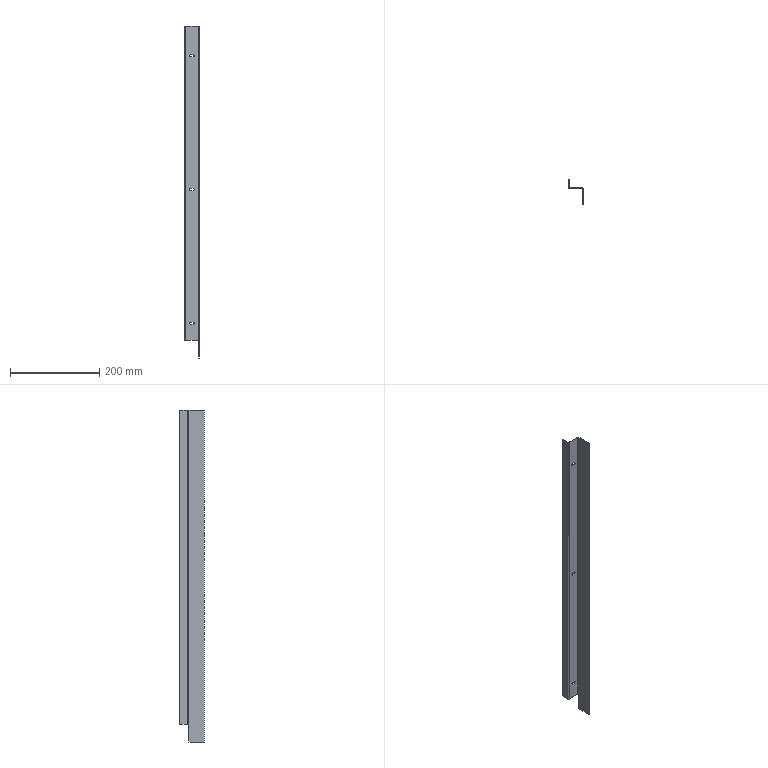Part | NX | features solid 2 | 1 solid | 31 faces | box 32.2 x 56 x 745 mm | volume 73805 mm3 | plane 18 | cylinder 13 | commonest cylinder face diameters 5 x9 2.4 x2 4.8 x2
STEP:
#1=CARTESIAN_POINT('',(1128.5,-1540.,1141.));
#2=VERTEX_POINT('',#1);
#3=CARTESIAN_POINT('',(1128.5,-1538.8,1141.));
#4=VERTEX_POINT('',#3);
#5=CARTESIAN_POINT('',(1128.5,-2286.595,1141.));
#6=DIRECTION('',(0.,1.,0.));
#7=VECTOR('',#6,1000.);
#8=LINE('',#5,#7);
#9=EDGE_CURVE('',#2,#4,#8,.T.);
#10=ORIENTED_EDGE('',*,*,#9,.T.);
#11=CARTESIAN_POINT('',(1123.5,-1538.8,1141.));
#12=VERTEX_POINT('',#11);
#13=CARTESIAN_POINT('',(1128.5,-1538.8,1141.));
#14=DIRECTION('',(-1.,0.,0.));
#15=VECTOR('',#14,1000.);
#16=LINE('',#13,#15);
#17=EDGE_CURVE('',#4,#12,#16,.T.);
#18=ORIENTED_EDGE('',*,*,#17,.T.);
#19=CARTESIAN_POINT('',(1123.5,-1540.,1141.));
#20=VERTEX_POINT('',#19);
#21=CARTESIAN_POINT('',(1123.5,-2286.595,1141.));
#22=DIRECTION('',(0.,1.,0.));
#23=VECTOR('',#22,1000.);
#24=LINE('',#21,#23);
#25=EDGE_CURVE('',#20,#12,#24,.T.);
#26=ORIENTED_EDGE('',*,*,#25,.F.);
#27=CARTESIAN_POINT('',(1141.,-1540.,1141.));
#28=DIRECTION('',(-1.,0.,0.));
#29=VECTOR('',#28,1000.);
#30=LINE('',#27,#29);
#31=EDGE_CURVE('',#2,#20,#30,.T.);
#32=ORIENTED_EDGE('',*,*,#31,.F.);
#33=EDGE_LOOP('',(#10,#18,#26,#32));
#34=FACE_BOUND('',#33,.T.);
#35=CARTESIAN_POINT('',(1128.5,-2286.595,1141.));
#36=DIRECTION('',(0.,0.,-1.));
#37=DIRECTION('',(0.,-1.,0.));
#38=AXIS2_PLACEMENT_3D('',#35,#36,#37);
#39=PLANE('',#38);
#40=ADVANCED_FACE('',(#34),#39,.F.);
#41=CARTESIAN_POINT('',(1128.5,-1540.,1146.));
#42=VERTEX_POINT('',#41);
#43=CARTESIAN_POINT('',(1128.5,-1538.8,1146.));
#44=VERTEX_POINT('',#43);
#45=CARTESIAN_POINT('',(1128.5,-2286.595,1146.));
#46=DIRECTION('',(0.,1.,0.));
#47=VECTOR('',#46,1000.);
#48=LINE('',#45,#47);
#49=EDGE_CURVE('',#42,#44,#48,.T.);
#50=ORIENTED_EDGE('',*,*,#49,.T.);
#51=CARTESIAN_POINT('',(1128.5,-1538.8,1143.5));
#52=DIRECTION('',(0.,1.,0.));
#53=DIRECTION('',(-1.,0.,0.));
#54=AXIS2_PLACEMENT_3D('',#51,#52,#53);
#55=CIRCLE('',#54,2.5);
#56=EDGE_CURVE('',#44,#4,#55,.T.);
#57=ORIENTED_EDGE('',*,*,#56,.T.);
#58=ORIENTED_EDGE('',*,*,#9,.F.);
#59=CARTESIAN_POINT('',(1128.5,-1540.,1143.5));
#60=DIRECTION('',(0.,1.,0.));
#61=DIRECTION('',(-1.,0.,0.));
#62=AXIS2_PLACEMENT_3D('',#59,#60,#61);
#63=CIRCLE('',#62,2.5);
#64=EDGE_CURVE('',#42,#2,#63,.T.);
#65=ORIENTED_EDGE('',*,*,#64,.F.);
#66=EDGE_LOOP('',(#50,#57,#58,#65));
#67=FACE_BOUND('',#66,.T.);
#68=CARTESIAN_POINT('',(1128.5,-2286.595,1143.5));
#69=DIRECTION('',(0.,1.,0.));
#70=DIRECTION('',(-1.,0.,0.));
#71=AXIS2_PLACEMENT_3D('',#68,#69,#70);
#72=CYLINDRICAL_SURFACE('',#71,2.5);
#73=ADVANCED_FACE('',(#67),#72,.F.);
#74=CARTESIAN_POINT('',(1123.5,-1540.,1146.));
#75=VERTEX_POINT('',#74);
#76=CARTESIAN_POINT('',(1123.5,-1538.8,1146.));
#77=VERTEX_POINT('',#76);
#78=CARTESIAN_POINT('',(1123.5,-2286.595,1146.));
#79=DIRECTION('',(0.,1.,0.));
#80=VECTOR('',#79,1000.);
#81=LINE('',#78,#80);
#82=EDGE_CURVE('',#75,#77,#81,.T.);
#83=ORIENTED_EDGE('',*,*,#82,.T.);
#84=CARTESIAN_POINT('',(1128.5,-1538.8,1146.));
#85=DIRECTION('',(1.,0.,0.));
#86=VECTOR('',#85,1000.);
#87=LINE('',#84,#86);
#88=EDGE_CURVE('',#77,#44,#87,.T.);
#89=ORIENTED_EDGE('',*,*,#88,.T.);
#90=ORIENTED_EDGE('',*,*,#49,.F.);
#91=CARTESIAN_POINT('',(1141.,-1540.,1146.));
#92=DIRECTION('',(1.,0.,0.));
#93=VECTOR('',#92,1000.);
#94=LINE('',#91,#93);
#95=EDGE_CURVE('',#75,#42,#94,.T.);
#96=ORIENTED_EDGE('',*,*,#95,.F.);
#97=EDGE_LOOP('',(#83,#89,#90,#96));
#98=FACE_BOUND('',#97,.T.);
#99=CARTESIAN_POINT('',(1128.5,-2286.595,1146.));
#100=DIRECTION('',(0.,0.,1.));
#101=DIRECTION('',(1.,0.,0.));
#102=AXIS2_PLACEMENT_3D('',#99,#100,#101);
#103=PLANE('',#102);
#104=ADVANCED_FACE('',(#98),#103,.F.);
#105=CARTESIAN_POINT('',(1121.,-1540.,1143.5));
#106=VERTEX_POINT('',#105);
#107=CARTESIAN_POINT('',(1121.,-1538.8,1143.5));
#108=VERTEX_POINT('',#107);
#109=CARTESIAN_POINT('',(1121.,-2286.595,1143.5));
#110=DIRECTION('',(0.,1.,0.));
#111=VECTOR('',#110,1000.);
#112=LINE('',#109,#111);
#113=EDGE_CURVE('',#106,#108,#112,.T.);
#114=ORIENTED_EDGE('',*,*,#113,.F.);
#115=CARTESIAN_POINT('',(1123.5,-1540.,1143.5));
#116=DIRECTION('',(0.,1.,0.));
#117=DIRECTION('',(-1.,0.,0.));
#118=AXIS2_PLACEMENT_3D('',#115,#116,#117);
#119=CIRCLE('',#118,2.5);
#120=EDGE_CURVE('',#20,#106,#119,.T.);
#121=ORIENTED_EDGE('',*,*,#120,.F.);
#122=ORIENTED_EDGE('',*,*,#25,.T.);
#123=CARTESIAN_POINT('',(1123.5,-1538.8,1143.5));
#124=DIRECTION('',(0.,1.,0.));
#125=DIRECTION('',(1.,0.,0.));
#126=AXIS2_PLACEMENT_3D('',#123,#124,#125);
#127=CIRCLE('',#126,2.5);
#128=EDGE_CURVE('',#12,#108,#127,.T.);
#129=ORIENTED_EDGE('',*,*,#128,.T.);
#130=EDGE_LOOP('',(#114,#121,#122,#129));
#131=FACE_BOUND('',#130,.T.);
#132=CARTESIAN_POINT('',(1123.5,-2286.595,1143.5));
#133=DIRECTION('',(0.,1.,0.));
#134=DIRECTION('',(-1.,0.,0.));
#135=AXIS2_PLACEMENT_3D('',#132,#133,#134);
#136=CYLINDRICAL_SURFACE('',#135,2.5);
#137=ADVANCED_FACE('',(#131),#136,.F.);
#138=CARTESIAN_POINT('',(1128.5,-1540.,841.));
#139=VERTEX_POINT('',#138);
#140=CARTESIAN_POINT('',(1128.5,-1538.8,841.));
#141=VERTEX_POINT('',#140);
#142=CARTESIAN_POINT('',(1128.5,-2286.595,841.));
#143=DIRECTION('',(0.,1.,0.));
#144=VECTOR('',#143,1000.);
#145=LINE('',#142,#144);
#146=EDGE_CURVE('',#139,#141,#145,.T.);
#147=ORIENTED_EDGE('',*,*,#146,.T.);
#148=CARTESIAN_POINT('',(1123.5,-1538.8,841.));
#149=VERTEX_POINT('',#148);
#150=CARTESIAN_POINT('',(1128.5,-1538.8,841.));
#151=DIRECTION('',(-1.,0.,0.));
#152=VECTOR('',#151,1000.);
#153=LINE('',#150,#152);
#154=EDGE_CURVE('',#141,#149,#153,.T.);
#155=ORIENTED_EDGE('',*,*,#154,.T.);
#156=CARTESIAN_POINT('',(1123.5,-1540.,841.));
#157=VERTEX_POINT('',#156);
#158=CARTESIAN_POINT('',(1123.5,-2286.595,841.));
#159=DIRECTION('',(0.,1.,0.));
#160=VECTOR('',#159,1000.);
#161=LINE('',#158,#160);
#162=EDGE_CURVE('',#157,#149,#161,.T.);
#163=ORIENTED_EDGE('',*,*,#162,.F.);
#164=CARTESIAN_POINT('',(1141.,-1540.,841.));
#165=DIRECTION('',(-1.,0.,0.));
#166=VECTOR('',#165,1000.);
#167=LINE('',#164,#166);
#168=EDGE_CURVE('',#139,#157,#167,.T.);
#169=ORIENTED_EDGE('',*,*,#168,.F.);
#170=EDGE_LOOP('',(#147,#155,#163,#169));
#171=FACE_BOUND('',#170,.T.);
#172=CARTESIAN_POINT('',(1128.5,-2286.595,841.));
#173=DIRECTION('',(0.,0.,-1.));
#174=DIRECTION('',(0.,-1.,0.));
#175=AXIS2_PLACEMENT_3D('',#172,#173,#174);
#176=PLANE('',#175);
#177=ADVANCED_FACE('',(#171),#176,.F.);
#178=CARTESIAN_POINT('',(1128.5,-1540.,846.));
#179=VERTEX_POINT('',#178);
#180=CARTESIAN_POINT('',(1128.5,-1538.8,846.));
#181=VERTEX_POINT('',#180);
#182=CARTESIAN_POINT('',(1128.5,-2286.595,846.));
#183=DIRECTION('',(0.,1.,0.));
#184=VECTOR('',#183,1000.);
#185=LINE('',#182,#184);
#186=EDGE_CURVE('',#179,#181,#185,.T.);
#187=ORIENTED_EDGE('',*,*,#186,.T.);
#188=CARTESIAN_POINT('',(1128.5,-1538.8,843.5));
#189=DIRECTION('',(0.,1.,0.));
#190=DIRECTION('',(0.,0.,1.));
#191=AXIS2_PLACEMENT_3D('',#188,#189,#190);
#192=CIRCLE('',#191,2.5);
#193=EDGE_CURVE('',#181,#141,#192,.T.);
#194=ORIENTED_EDGE('',*,*,#193,.T.);
#195=ORIENTED_EDGE('',*,*,#146,.F.);
#196=CARTESIAN_POINT('',(1128.5,-1540.,843.5));
#197=DIRECTION('',(0.,1.,0.));
#198=DIRECTION('',(-1.,0.,0.));
#199=AXIS2_PLACEMENT_3D('',#196,#197,#198);
#200=CIRCLE('',#199,2.5);
#201=EDGE_CURVE('',#179,#139,#200,.T.);
#202=ORIENTED_EDGE('',*,*,#201,.F.);
#203=EDGE_LOOP('',(#187,#194,#195,#202));
#204=FACE_BOUND('',#203,.T.);
#205=CARTESIAN_POINT('',(1128.5,-2286.595,843.5));
#206=DIRECTION('',(0.,1.,0.));
#207=DIRECTION('',(-1.,0.,0.));
#208=AXIS2_PLACEMENT_3D('',#205,#206,#207);
#209=CYLINDRICAL_SURFACE('',#208,2.5);
#210=ADVANCED_FACE('',(#204),#209,.F.);
#211=CARTESIAN_POINT('',(1123.5,-1540.,846.));
#212=VERTEX_POINT('',#211);
#213=CARTESIAN_POINT('',(1123.5,-1538.8,846.));
#214=VERTEX_POINT('',#213);
#215=CARTESIAN_POINT('',(1123.5,-2286.595,846.));
#216=DIRECTION('',(0.,1.,0.));
#217=VECTOR('',#216,1000.);
#218=LINE('',#215,#217);
#219=EDGE_CURVE('',#212,#214,#218,.T.);
#220=ORIENTED_EDGE('',*,*,#219,.T.);
#221=CARTESIAN_POINT('',(1128.5,-1538.8,846.));
#222=DIRECTION('',(1.,0.,0.));
#223=VECTOR('',#222,1000.);
#224=LINE('',#221,#223);
#225=EDGE_CURVE('',#214,#181,#224,.T.);
#226=ORIENTED_EDGE('',*,*,#225,.T.);
#227=ORIENTED_EDGE('',*,*,#186,.F.);
#228=CARTESIAN_POINT('',(1141.,-1540.,846.));
#229=DIRECTION('',(1.,0.,0.));
#230=VECTOR('',#229,1000.);
#231=LINE('',#228,#230);
#232=EDGE_CURVE('',#212,#179,#231,.T.);
#233=ORIENTED_EDGE('',*,*,#232,.F.);
#234=EDGE_LOOP('',(#220,#226,#227,#233));
#235=FACE_BOUND('',#234,.T.);
#236=CARTESIAN_POINT('',(1128.5,-2286.595,846.));
#237=DIRECTION('',(0.,0.,1.));
#238=DIRECTION('',(1.,0.,0.));
#239=AXIS2_PLACEMENT_3D('',#236,#237,#238);
#240=PLANE('',#239);
#241=ADVANCED_FACE('',(#235),#240,.F.);
#242=CARTESIAN_POINT('',(1121.,-1540.,843.5));
#243=VERTEX_POINT('',#242);
#244=CARTESIAN_POINT('',(1121.,-1538.8,843.5));
#245=VERTEX_POINT('',#244);
#246=CARTESIAN_POINT('',(1121.,-2286.595,843.5));
#247=DIRECTION('',(0.,1.,0.));
#248=VECTOR('',#247,1000.);
#249=LINE('',#246,#248);
#250=EDGE_CURVE('',#243,#245,#249,.T.);
#251=ORIENTED_EDGE('',*,*,#250,.F.);
#252=CARTESIAN_POINT('',(1123.5,-1540.,843.5));
#253=DIRECTION('',(0.,1.,0.));
#254=DIRECTION('',(-1.,0.,0.));
#255=AXIS2_PLACEMENT_3D('',#252,#253,#254);
#256=CIRCLE('',#255,2.5);
#257=EDGE_CURVE('',#157,#243,#256,.T.);
#258=ORIENTED_EDGE('',*,*,#257,.F.);
#259=ORIENTED_EDGE('',*,*,#162,.T.);
#260=CARTESIAN_POINT('',(1123.5,-1538.8,843.5));
#261=DIRECTION('',(0.,1.,0.));
#262=DIRECTION('',(0.,0.,-1.));
#263=AXIS2_PLACEMENT_3D('',#260,#261,#262);
#264=CIRCLE('',#263,2.5);
#265=EDGE_CURVE('',#149,#245,#264,.T.);
#266=ORIENTED_EDGE('',*,*,#265,.T.);
#267=EDGE_LOOP('',(#251,#258,#259,#266));
#268=FACE_BOUND('',#267,.T.);
#269=CARTESIAN_POINT('',(1123.5,-2286.595,843.5));
#270=DIRECTION('',(0.,1.,0.));
#271=DIRECTION('',(-1.,0.,0.));
#272=AXIS2_PLACEMENT_3D('',#269,#270,#271);
#273=CYLINDRICAL_SURFACE('',#272,2.5);
#274=ADVANCED_FACE('',(#268),#273,.F.);
#275=CARTESIAN_POINT('',(1128.5,-1540.,541.));
#276=VERTEX_POINT('',#275);
#277=CARTESIAN_POINT('',(1128.5,-1538.8,541.));
#278=VERTEX_POINT('',#277);
#279=CARTESIAN_POINT('',(1128.5,-2286.595,541.));
#280=DIRECTION('',(0.,1.,0.));
#281=VECTOR('',#280,1000.);
#282=LINE('',#279,#281);
#283=EDGE_CURVE('',#276,#278,#282,.T.);
#284=ORIENTED_EDGE('',*,*,#283,.T.);
#285=CARTESIAN_POINT('',(1123.5,-1538.8,541.));
#286=VERTEX_POINT('',#285);
#287=CARTESIAN_POINT('',(1128.5,-1538.8,541.));
#288=DIRECTION('',(-1.,0.,0.));
#289=VECTOR('',#288,1000.);
#290=LINE('',#287,#289);
#291=EDGE_CURVE('',#278,#286,#290,.T.);
#292=ORIENTED_EDGE('',*,*,#291,.T.);
#293=CARTESIAN_POINT('',(1123.5,-1540.,541.));
#294=VERTEX_POINT('',#293);
#295=CARTESIAN_POINT('',(1123.5,-2286.595,541.));
#296=DIRECTION('',(0.,1.,0.));
#297=VECTOR('',#296,1000.);
#298=LINE('',#295,#297);
#299=EDGE_CURVE('',#294,#286,#298,.T.);
#300=ORIENTED_EDGE('',*,*,#299,.F.);
#301=CARTESIAN_POINT('',(1141.,-1540.,541.));
#302=DIRECTION('',(-1.,0.,0.));
#303=VECTOR('',#302,1000.);
#304=LINE('',#301,#303);
#305=EDGE_CURVE('',#276,#294,#304,.T.);
#306=ORIENTED_EDGE('',*,*,#305,.F.);
#307=EDGE_LOOP('',(#284,#292,#300,#306));
#308=FACE_BOUND('',#307,.T.);
#309=CARTESIAN_POINT('',(1128.5,-2286.595,541.));
#310=DIRECTION('',(0.,0.,-1.));
#311=DIRECTION('',(0.,-1.,0.));
#312=AXIS2_PLACEMENT_3D('',#309,#310,#311);
#313=PLANE('',#312);
#314=ADVANCED_FACE('',(#308),#313,.F.);
#315=CARTESIAN_POINT('',(1128.5,-1540.,546.));
#316=VERTEX_POINT('',#315);
#317=CARTESIAN_POINT('',(1128.5,-1538.8,546.));
#318=VERTEX_POINT('',#317);
#319=CARTESIAN_POINT('',(1128.5,-2286.595,546.));
#320=DIRECTION('',(0.,1.,0.));
#321=VECTOR('',#320,1000.);
#322=LINE('',#319,#321);
#323=EDGE_CURVE('',#316,#318,#322,.T.);
#324=ORIENTED_EDGE('',*,*,#323,.T.);
#325=CARTESIAN_POINT('',(1128.5,-1538.8,543.5));
#326=DIRECTION('',(0.,1.,0.));
#327=DIRECTION('',(-1.,0.,0.));
#328=AXIS2_PLACEMENT_3D('',#325,#326,#327);
#329=CIRCLE('',#328,2.5);
#330=EDGE_CURVE('',#318,#278,#329,.T.);
#331=ORIENTED_EDGE('',*,*,#330,.T.);
#332=ORIENTED_EDGE('',*,*,#283,.F.);
#333=CARTESIAN_POINT('',(1128.5,-1540.,543.5));
#334=DIRECTION('',(0.,1.,0.));
#335=DIRECTION('',(-1.,0.,0.));
#336=AXIS2_PLACEMENT_3D('',#333,#334,#335);
#337=CIRCLE('',#336,2.5);
#338=EDGE_CURVE('',#316,#276,#337,.T.);
#339=ORIENTED_EDGE('',*,*,#338,.F.);
#340=EDGE_LOOP('',(#324,#331,#332,#339));
#341=FACE_BOUND('',#340,.T.);
#342=CARTESIAN_POINT('',(1128.5,-2286.595,543.5));
#343=DIRECTION('',(0.,1.,0.));
#344=DIRECTION('',(-1.,0.,0.));
#345=AXIS2_PLACEMENT_3D('',#342,#343,#344);
#346=CYLINDRICAL_SURFACE('',#345,2.5);
#347=ADVANCED_FACE('',(#341),#346,.F.);
#348=CARTESIAN_POINT('',(1123.5,-1540.,546.));
#349=VERTEX_POINT('',#348);
#350=CARTESIAN_POINT('',(1123.5,-1538.8,546.));
#351=VERTEX_POINT('',#350);
#352=CARTESIAN_POINT('',(1123.5,-2286.595,546.));
#353=DIRECTION('',(0.,1.,0.));
#354=VECTOR('',#353,1000.);
#355=LINE('',#352,#354);
#356=EDGE_CURVE('',#349,#351,#355,.T.);
#357=ORIENTED_EDGE('',*,*,#356,.T.);
#358=CARTESIAN_POINT('',(1128.5,-1538.8,546.));
#359=DIRECTION('',(1.,0.,0.));
#360=VECTOR('',#359,1000.);
#361=LINE('',#358,#360);
#362=EDGE_CURVE('',#351,#318,#361,.T.);
#363=ORIENTED_EDGE('',*,*,#362,.T.);
#364=ORIENTED_EDGE('',*,*,#323,.F.);
#365=CARTESIAN_POINT('',(1141.,-1540.,546.));
#366=DIRECTION('',(1.,0.,0.));
#367=VECTOR('',#366,1000.);
#368=LINE('',#365,#367);
#369=EDGE_CURVE('',#349,#316,#368,.T.);
#370=ORIENTED_EDGE('',*,*,#369,.F.);
#371=EDGE_LOOP('',(#357,#363,#364,#370));
#372=FACE_BOUND('',#371,.T.);
#373=CARTESIAN_POINT('',(1128.5,-2286.595,546.));
#374=DIRECTION('',(0.,0.,1.));
#375=DIRECTION('',(1.,0.,0.));
#376=AXIS2_PLACEMENT_3D('',#373,#374,#375);
#377=PLANE('',#376);
#378=ADVANCED_FACE('',(#372),#377,.F.);
#379=CARTESIAN_POINT('',(1121.,-1540.,543.5));
#380=VERTEX_POINT('',#379);
#381=CARTESIAN_POINT('',(1121.,-1538.8,543.5));
#382=VERTEX_POINT('',#381);
#383=CARTESIAN_POINT('',(1121.,-2286.595,543.5));
#384=DIRECTION('',(0.,1.,0.));
#385=VECTOR('',#384,1000.);
#386=LINE('',#383,#385);
#387=EDGE_CURVE('',#380,#382,#386,.T.);
#388=ORIENTED_EDGE('',*,*,#387,.F.);
#389=CARTESIAN_POINT('',(1123.5,-1540.,543.5));
#390=DIRECTION('',(0.,1.,0.));
#391=DIRECTION('',(-1.,0.,0.));
#392=AXIS2_PLACEMENT_3D('',#389,#390,#391);
#393=CIRCLE('',#392,2.5);
#394=EDGE_CURVE('',#294,#380,#393,.T.);
#395=ORIENTED_EDGE('',*,*,#394,.F.);
#396=ORIENTED_EDGE('',*,*,#299,.T.);
#397=CARTESIAN_POINT('',(1123.5,-1538.8,543.5));
#398=DIRECTION('',(0.,1.,0.));
#399=DIRECTION('',(1.,0.,0.));
#400=AXIS2_PLACEMENT_3D('',#397,#398,#399);
#401=CIRCLE('',#400,2.5);
#402=EDGE_CURVE('',#286,#382,#401,.T.);
#403=ORIENTED_EDGE('',*,*,#402,.T.);
#404=EDGE_LOOP('',(#388,#395,#396,#403));
#405=FACE_BOUND('',#404,.T.);
#406=CARTESIAN_POINT('',(1123.5,-2286.595,543.5));
#407=DIRECTION('',(0.,1.,0.));
#408=DIRECTION('',(-1.,0.,0.));
#409=AXIS2_PLACEMENT_3D('',#406,#407,#408);
#410=CYLINDRICAL_SURFACE('',#409,2.5);
#411=ADVANCED_FACE('',(#405),#410,.F.);
#412=CARTESIAN_POINT('',(1110.,-1537.6,505.5));
#413=VERTEX_POINT('',#412);
#414=CARTESIAN_POINT('',(1110.,-1520.,505.5));
#415=VERTEX_POINT('',#414);
#416=CARTESIAN_POINT('',(1110.,-1540.,505.5));
#417=DIRECTION('',(0.,1.,0.));
#418=VECTOR('',#417,1000.);
#419=LINE('',#416,#418);
#420=EDGE_CURVE('',#413,#415,#419,.T.);
#421=ORIENTED_EDGE('',*,*,#420,.T.);
#422=CARTESIAN_POINT('',(1111.2,-1520.,505.5));
#423=VERTEX_POINT('',#422);
#424=CARTESIAN_POINT('',(1110.,-1520.,505.5));
#425=DIRECTION('',(-1.,0.,0.));
#426=VECTOR('',#425,1000.);
#427=LINE('',#424,#426);
#428=EDGE_CURVE('',#423,#415,#427,.T.);
#429=ORIENTED_EDGE('',*,*,#428,.F.);
#430=CARTESIAN_POINT('',(1111.2,-1537.6,505.5));
#431=VERTEX_POINT('',#430);
#432=CARTESIAN_POINT('',(1111.2,-1540.,505.5));
#433=DIRECTION('',(0.,1.,0.));
#434=VECTOR('',#433,1000.);
#435=LINE('',#432,#434);
#436=EDGE_CURVE('',#431,#423,#435,.T.);
#437=ORIENTED_EDGE('',*,*,#436,.F.);
#438=CARTESIAN_POINT('',(1112.4,-1538.8,505.5));
#439=VERTEX_POINT('',#438);
#440=CARTESIAN_POINT('',(1112.4,-1537.6,505.5));
#441=DIRECTION('',(0.,0.,-1.));
#442=DIRECTION('',(-1.,0.,0.));
#443=AXIS2_PLACEMENT_3D('',#440,#441,#442);
#444=CIRCLE('',#443,1.2);
#445=EDGE_CURVE('',#439,#431,#444,.T.);
#446=ORIENTED_EDGE('',*,*,#445,.F.);
#447=CARTESIAN_POINT('',(1139.8,-1538.8,505.5));
#448=VERTEX_POINT('',#447);
#449=CARTESIAN_POINT('',(1141.,-1538.8,505.5));
#450=DIRECTION('',(-1.,0.,0.));
#451=VECTOR('',#450,1000.);
#452=LINE('',#449,#451);
#453=EDGE_CURVE('',#448,#439,#452,.T.);
#454=ORIENTED_EDGE('',*,*,#453,.F.);
#455=CARTESIAN_POINT('',(1142.2,-1541.2,505.5));
#456=VERTEX_POINT('',#455);
#457=CARTESIAN_POINT('',(1139.8,-1541.2,505.5));
#458=DIRECTION('',(0.,0.,1.));
#459=DIRECTION('',(-1.,0.,0.));
#460=AXIS2_PLACEMENT_3D('',#457,#458,#459);
#461=CIRCLE('',#460,2.4);
#462=EDGE_CURVE('',#456,#448,#461,.T.);
#463=ORIENTED_EDGE('',*,*,#462,.F.);
#464=CARTESIAN_POINT('',(1141.,-1541.2,505.5));
#465=VERTEX_POINT('',#464);
#466=CARTESIAN_POINT('',(1141.,-1541.2,505.5));
#467=DIRECTION('',(-1.,0.,0.));
#468=VECTOR('',#467,1000.);
#469=LINE('',#466,#468);
#470=EDGE_CURVE('',#456,#465,#469,.T.);
#471=ORIENTED_EDGE('',*,*,#470,.T.);
#472=CARTESIAN_POINT('',(1139.8,-1540.,505.5));
#473=VERTEX_POINT('',#472);
#474=CARTESIAN_POINT('',(1139.8,-1541.2,505.5));
#475=DIRECTION('',(0.,0.,1.));
#476=DIRECTION('',(1.,0.,0.));
#477=AXIS2_PLACEMENT_3D('',#474,#475,#476);
#478=CIRCLE('',#477,1.2);
#479=EDGE_CURVE('',#465,#473,#478,.T.);
#480=ORIENTED_EDGE('',*,*,#479,.T.);
#481=CARTESIAN_POINT('',(1112.4,-1540.,505.5));
#482=VERTEX_POINT('',#481);
#483=CARTESIAN_POINT('',(1141.,-1540.,505.5));
#484=DIRECTION('',(-1.,0.,0.));
#485=VECTOR('',#484,1000.);
#486=LINE('',#483,#485);
#487=EDGE_CURVE('',#473,#482,#486,.T.);
#488=ORIENTED_EDGE('',*,*,#487,.T.);
#489=CARTESIAN_POINT('',(1112.4,-1537.6,505.5));
#490=DIRECTION('',(0.,0.,-1.));
#491=DIRECTION('',(1.,0.,0.));
#492=AXIS2_PLACEMENT_3D('',#489,#490,#491);
#493=CIRCLE('',#492,2.4);
#494=EDGE_CURVE('',#482,#413,#493,.T.);
#495=ORIENTED_EDGE('',*,*,#494,.T.);
#496=EDGE_LOOP('',(#421,#429,#437,#446,#454,#463,#471,#480,#488,#495));
#497=FACE_BOUND('',#496,.T.);
#498=CARTESIAN_POINT('',(1110.,-1540.,505.5));
#499=DIRECTION('',(0.,0.,-1.));
#500=DIRECTION('',(0.,-1.,0.));
#501=AXIS2_PLACEMENT_3D('',#498,#499,#500);
#502=PLANE('',#501);
#503=ADVANCED_FACE('',(#497),#502,.T.);
#504=CARTESIAN_POINT('',(1142.2,-1541.2,465.5));
#505=VERTEX_POINT('',#504);
#506=CARTESIAN_POINT('',(1141.,-1541.2,465.5));
#507=VERTEX_POINT('',#506);
#508=CARTESIAN_POINT('',(1141.,-1541.2,465.5));
#509=DIRECTION('',(-1.,0.,0.));
#510=VECTOR('',#509,1000.);
#511=LINE('',#508,#510);
#512=EDGE_CURVE('',#505,#507,#511,.T.);
#513=ORIENTED_EDGE('',*,*,#512,.T.);
#514=CARTESIAN_POINT('',(1141.,-1541.2,465.5));
#515=DIRECTION('',(0.,0.,1.));
#516=VECTOR('',#515,1000.);
#517=LINE('',#514,#516);
#518=EDGE_CURVE('',#507,#465,#517,.T.);
#519=ORIENTED_EDGE('',*,*,#518,.T.);
#520=ORIENTED_EDGE('',*,*,#470,.F.);
#521=CARTESIAN_POINT('',(1142.2,-1541.2,465.5));
#522=DIRECTION('',(0.,0.,1.));
#523=VECTOR('',#522,1000.);
#524=LINE('',#521,#523);
#525=EDGE_CURVE('',#505,#456,#524,.T.);
#526=ORIENTED_EDGE('',*,*,#525,.F.);
#527=EDGE_LOOP('',(#513,#519,#520,#526));
#528=FACE_BOUND('',#527,.T.);
#529=CARTESIAN_POINT('',(1141.,-1541.2,485.5));
#530=DIRECTION('',(0.,1.,0.));
#531=DIRECTION('',(1.,0.,0.));
#532=AXIS2_PLACEMENT_3D('',#529,#530,#531);
#533=PLANE('',#532);
#534=ADVANCED_FACE('',(#528),#533,.T.);
#535=CARTESIAN_POINT('',(1110.,-1520.,1210.5));
#536=VERTEX_POINT('',#535);
#537=CARTESIAN_POINT('',(1110.,-1520.,465.5));
#538=DIRECTION('',(0.,0.,1.));
#539=VECTOR('',#538,1000.);
#540=LINE('',#537,#539);
#541=EDGE_CURVE('',#415,#536,#540,.T.);
#542=ORIENTED_EDGE('',*,*,#541,.F.);
#543=ORIENTED_EDGE('',*,*,#420,.F.);
#544=CARTESIAN_POINT('',(1110.,-1537.6,1210.5));
#545=VERTEX_POINT('',#544);
#546=CARTESIAN_POINT('',(1110.,-1537.6,465.5));
#547=DIRECTION('',(0.,0.,1.));
#548=VECTOR('',#547,1000.);
#549=LINE('',#546,#548);
#550=EDGE_CURVE('',#413,#545,#549,.T.);
#551=ORIENTED_EDGE('',*,*,#550,.T.);
#552=CARTESIAN_POINT('',(1110.,-1540.,1210.5));
#553=DIRECTION('',(0.,1.,0.));
#554=VECTOR('',#553,1000.);
#555=LINE('',#552,#554);
#556=EDGE_CURVE('',#545,#536,#555,.T.);
#557=ORIENTED_EDGE('',*,*,#556,.T.);
#558=EDGE_LOOP('',(#542,#543,#551,#557));
#559=FACE_BOUND('',#558,.T.);
#560=CARTESIAN_POINT('',(1110.,-1540.,465.5));
#561=DIRECTION('',(1.,0.,0.));
#562=DIRECTION('',(0.,0.,1.));
#563=AXIS2_PLACEMENT_3D('',#560,#561,#562);
#564=PLANE('',#563);
#565=ADVANCED_FACE('',(#559),#564,.F.);
#566=ORIENTED_EDGE('',*,*,#550,.F.);
#567=ORIENTED_EDGE('',*,*,#494,.F.);
#568=CARTESIAN_POINT('',(1112.4,-1540.,1210.5));
#569=VERTEX_POINT('',#568);
#570=CARTESIAN_POINT('',(1112.4,-1540.,465.5));
#571=DIRECTION('',(0.,0.,1.));
#572=VECTOR('',#571,1000.);
#573=LINE('',#570,#572);
#574=EDGE_CURVE('',#482,#569,#573,.T.);
#575=ORIENTED_EDGE('',*,*,#574,.T.);
#576=CARTESIAN_POINT('',(1112.4,-1537.6,1210.5));
#577=DIRECTION('',(0.,0.,-1.));
#578=DIRECTION('',(-1.,0.,0.));
#579=AXIS2_PLACEMENT_3D('',#576,#577,#578);
#580=CIRCLE('',#579,2.4);
#581=EDGE_CURVE('',#569,#545,#580,.T.);
#582=ORIENTED_EDGE('',*,*,#581,.T.);
#583=EDGE_LOOP('',(#566,#567,#575,#582));
#584=FACE_BOUND('',#583,.T.);
#585=CARTESIAN_POINT('',(1112.4,-1537.6,465.5));
#586=DIRECTION('',(0.,0.,1.));
#587=DIRECTION('',(-1.,0.,0.));
#588=AXIS2_PLACEMENT_3D('',#585,#586,#587);
#589=CYLINDRICAL_SURFACE('',#588,2.4);
#590=ADVANCED_FACE('',(#584),#589,.T.);
#591=ORIENTED_EDGE('',*,*,#305,.T.);
#592=ORIENTED_EDGE('',*,*,#394,.T.);
#593=CARTESIAN_POINT('',(1123.5,-1540.,543.5));
#594=DIRECTION('',(0.,1.,0.));
#595=DIRECTION('',(-1.,0.,0.));
#596=AXIS2_PLACEMENT_3D('',#593,#594,#595);
#597=CIRCLE('',#596,2.5);
#598=EDGE_CURVE('',#380,#349,#597,.T.);
#599=ORIENTED_EDGE('',*,*,#598,.T.);
#600=ORIENTED_EDGE('',*,*,#369,.T.);
#601=ORIENTED_EDGE('',*,*,#338,.T.);
#602=EDGE_LOOP('',(#591,#592,#599,#600,#601));
#603=FACE_BOUND('',#602,.T.);
#604=ORIENTED_EDGE('',*,*,#168,.T.);
#605=ORIENTED_EDGE('',*,*,#257,.T.);
#606=CARTESIAN_POINT('',(1123.5,-1540.,843.5));
#607=DIRECTION('',(0.,1.,0.));
#608=DIRECTION('',(-1.,0.,0.));
#609=AXIS2_PLACEMENT_3D('',#606,#607,#608);
#610=CIRCLE('',#609,2.5);
#611=EDGE_CURVE('',#243,#212,#610,.T.);
#612=ORIENTED_EDGE('',*,*,#611,.T.);
#613=ORIENTED_EDGE('',*,*,#232,.T.);
#614=ORIENTED_EDGE('',*,*,#201,.T.);
#615=EDGE_LOOP('',(#604,#605,#612,#613,#614));
#616=FACE_BOUND('',#615,.T.);
#617=ORIENTED_EDGE('',*,*,#31,.T.);
#618=ORIENTED_EDGE('',*,*,#120,.T.);
#619=CARTESIAN_POINT('',(1123.5,-1540.,1143.5));
#620=DIRECTION('',(0.,1.,0.));
#621=DIRECTION('',(-1.,0.,0.));
#622=AXIS2_PLACEMENT_3D('',#619,#620,#621);
#623=CIRCLE('',#622,2.5);
#624=EDGE_CURVE('',#106,#75,#623,.T.);
#625=ORIENTED_EDGE('',*,*,#624,.T.);
#626=ORIENTED_EDGE('',*,*,#95,.T.);
#627=ORIENTED_EDGE('',*,*,#64,.T.);
#628=EDGE_LOOP('',(#617,#618,#625,#626,#627));
#629=FACE_BOUND('',#628,.T.);
#630=ORIENTED_EDGE('',*,*,#574,.F.);
#631=ORIENTED_EDGE('',*,*,#487,.F.);
#632=CARTESIAN_POINT('',(1139.8,-1540.,1210.5));
#633=VERTEX_POINT('',#632);
#634=CARTESIAN_POINT('',(1139.8,-1540.,465.5));
#635=DIRECTION('',(0.,0.,1.));
#636=VECTOR('',#635,1000.);
#637=LINE('',#634,#636);
#638=EDGE_CURVE('',#473,#633,#637,.T.);
#639=ORIENTED_EDGE('',*,*,#638,.T.);
#640=CARTESIAN_POINT('',(1141.,-1540.,1210.5));
#641=DIRECTION('',(-1.,0.,0.));
#642=VECTOR('',#641,1000.);
#643=LINE('',#640,#642);
#644=EDGE_CURVE('',#633,#569,#643,.T.);
#645=ORIENTED_EDGE('',*,*,#644,.T.);
#646=EDGE_LOOP('',(#630,#631,#639,#645));
#647=FACE_BOUND('',#646,.T.);
#648=CARTESIAN_POINT('',(1141.,-1540.,465.5));
#649=DIRECTION('',(0.,1.,0.));
#650=DIRECTION('',(1.,0.,0.));
#651=AXIS2_PLACEMENT_3D('',#648,#649,#650);
#652=PLANE('',#651);
#653=ADVANCED_FACE('',(#603,#616,#629,#647),#652,.F.);
#654=ORIENTED_EDGE('',*,*,#638,.F.);
#655=ORIENTED_EDGE('',*,*,#479,.F.);
#656=CARTESIAN_POINT('',(1141.,-1541.2,1210.5));
#657=VERTEX_POINT('',#656);
#658=CARTESIAN_POINT('',(1141.,-1541.2,465.5));
#659=DIRECTION('',(0.,0.,1.));
#660=VECTOR('',#659,1000.);
#661=LINE('',#658,#660);
#662=EDGE_CURVE('',#465,#657,#661,.T.);
#663=ORIENTED_EDGE('',*,*,#662,.T.);
#664=CARTESIAN_POINT('',(1139.8,-1541.2,1210.5));
#665=DIRECTION('',(0.,0.,1.));
#666=DIRECTION('',(1.,0.,0.));
#667=AXIS2_PLACEMENT_3D('',#664,#665,#666);
#668=CIRCLE('',#667,1.2);
#669=EDGE_CURVE('',#657,#633,#668,.T.);
#670=ORIENTED_EDGE('',*,*,#669,.T.);
#671=EDGE_LOOP('',(#654,#655,#663,#670));
#672=FACE_BOUND('',#671,.T.);
#673=CARTESIAN_POINT('',(1139.8,-1541.2,465.5));
#674=DIRECTION('',(0.,0.,1.));
#675=DIRECTION('',(-1.,0.,0.));
#676=AXIS2_PLACEMENT_3D('',#673,#674,#675);
#677=CYLINDRICAL_SURFACE('',#676,1.2);
#678=ADVANCED_FACE('',(#672),#677,.F.);
#679=CARTESIAN_POINT('',(1141.,-1576.,1210.5));
#680=VERTEX_POINT('',#679);
#681=CARTESIAN_POINT('',(1141.,-1576.,1210.5));
#682=DIRECTION('',(0.,1.,0.));
#683=VECTOR('',#682,1000.);
#684=LINE('',#681,#683);
#685=EDGE_CURVE('',#680,#657,#684,.T.);
#686=ORIENTED_EDGE('',*,*,#685,.T.);
#687=ORIENTED_EDGE('',*,*,#662,.F.);
#688=ORIENTED_EDGE('',*,*,#518,.F.);
#689=CARTESIAN_POINT('',(1141.,-1576.,465.5));
#690=VERTEX_POINT('',#689);
#691=CARTESIAN_POINT('',(1141.,-1576.,465.5));
#692=DIRECTION('',(0.,1.,0.));
#693=VECTOR('',#692,1000.);
#694=LINE('',#691,#693);
#695=EDGE_CURVE('',#690,#507,#694,.T.);
#696=ORIENTED_EDGE('',*,*,#695,.F.);
#697=CARTESIAN_POINT('',(1141.,-1576.,465.5));
#698=DIRECTION('',(0.,0.,1.));
#699=VECTOR('',#698,1000.);
#700=LINE('',#697,#699);
#701=EDGE_CURVE('',#690,#680,#700,.T.);
#702=ORIENTED_EDGE('',*,*,#701,.T.);
#703=EDGE_LOOP('',(#686,#687,#688,#696,#702));
#704=FACE_BOUND('',#703,.T.);
#705=CARTESIAN_POINT('',(1141.,-1576.,465.5));
#706=DIRECTION('',(1.,0.,0.));
#707=DIRECTION('',(0.,0.,1.));
#708=AXIS2_PLACEMENT_3D('',#705,#706,#707);
#709=PLANE('',#708);
#710=ADVANCED_FACE('',(#704),#709,.F.);
#711=ORIENTED_EDGE('',*,*,#436,.T.);
#712=CARTESIAN_POINT('',(1111.2,-1520.,1210.5));
#713=VERTEX_POINT('',#712);
#714=CARTESIAN_POINT('',(1111.2,-1520.,465.5));
#715=DIRECTION('',(0.,0.,1.));
#716=VECTOR('',#715,1000.);
#717=LINE('',#714,#716);
#718=EDGE_CURVE('',#423,#713,#717,.T.);
#719=ORIENTED_EDGE('',*,*,#718,.T.);
#720=CARTESIAN_POINT('',(1111.2,-1537.6,1210.5));
#721=VERTEX_POINT('',#720);
#722=CARTESIAN_POINT('',(1111.2,-1540.,1210.5));
#723=DIRECTION('',(0.,1.,0.));
#724=VECTOR('',#723,1000.);
#725=LINE('',#722,#724);
#726=EDGE_CURVE('',#721,#713,#725,.T.);
#727=ORIENTED_EDGE('',*,*,#726,.F.);
#728=CARTESIAN_POINT('',(1111.2,-1537.6,465.5));
#729=DIRECTION('',(0.,0.,1.));
#730=VECTOR('',#729,1000.);
#731=LINE('',#728,#730);
#732=EDGE_CURVE('',#431,#721,#731,.T.);
#733=ORIENTED_EDGE('',*,*,#732,.F.);
#734=EDGE_LOOP('',(#711,#719,#727,#733));
#735=FACE_BOUND('',#734,.T.);
#736=CARTESIAN_POINT('',(1111.2,-1540.,465.5));
#737=DIRECTION('',(1.,0.,0.));
#738=DIRECTION('',(0.,0.,1.));
#739=AXIS2_PLACEMENT_3D('',#736,#737,#738);
#740=PLANE('',#739);
#741=ADVANCED_FACE('',(#735),#740,.T.);
#742=ORIENTED_EDGE('',*,*,#445,.T.);
#743=ORIENTED_EDGE('',*,*,#732,.T.);
#744=CARTESIAN_POINT('',(1112.4,-1538.8,1210.5));
#745=VERTEX_POINT('',#744);
#746=CARTESIAN_POINT('',(1112.4,-1537.6,1210.5));
#747=DIRECTION('',(0.,0.,-1.));
#748=DIRECTION('',(-1.,0.,0.));
#749=AXIS2_PLACEMENT_3D('',#746,#747,#748);
#750=CIRCLE('',#749,1.2);
#751=EDGE_CURVE('',#745,#721,#750,.T.);
#752=ORIENTED_EDGE('',*,*,#751,.F.);
#753=CARTESIAN_POINT('',(1112.4,-1538.8,465.5));
#754=DIRECTION('',(0.,0.,1.));
#755=VECTOR('',#754,1000.);
#756=LINE('',#753,#755);
#757=EDGE_CURVE('',#439,#745,#756,.T.);
#758=ORIENTED_EDGE('',*,*,#757,.F.);
#759=EDGE_LOOP('',(#742,#743,#752,#758));
#760=FACE_BOUND('',#759,.T.);
#761=CARTESIAN_POINT('',(1112.4,-1537.6,465.5));
#762=DIRECTION('',(0.,0.,1.));
#763=DIRECTION('',(-1.,0.,0.));
#764=AXIS2_PLACEMENT_3D('',#761,#762,#763);
#765=CYLINDRICAL_SURFACE('',#764,1.2);
#766=ADVANCED_FACE('',(#760),#765,.F.);
#767=ORIENTED_EDGE('',*,*,#402,.F.);
#768=ORIENTED_EDGE('',*,*,#291,.F.);
#769=ORIENTED_EDGE('',*,*,#330,.F.);
#770=ORIENTED_EDGE('',*,*,#362,.F.);
#771=CARTESIAN_POINT('',(1123.5,-1538.8,543.5));
#772=DIRECTION('',(0.,1.,0.));
#773=DIRECTION('',(1.,0.,0.));
#774=AXIS2_PLACEMENT_3D('',#771,#772,#773);
#775=CIRCLE('',#774,2.5);
#776=EDGE_CURVE('',#382,#351,#775,.T.);
#777=ORIENTED_EDGE('',*,*,#776,.F.);
#778=EDGE_LOOP('',(#767,#768,#769,#770,#777));
#779=FACE_BOUND('',#778,.T.);
#780=ORIENTED_EDGE('',*,*,#265,.F.);
#781=ORIENTED_EDGE('',*,*,#154,.F.);
#782=ORIENTED_EDGE('',*,*,#193,.F.);
#783=ORIENTED_EDGE('',*,*,#225,.F.);
#784=CARTESIAN_POINT('',(1123.5,-1538.8,843.5));
#785=DIRECTION('',(0.,1.,0.));
#786=DIRECTION('',(0.,0.,-1.));
#787=AXIS2_PLACEMENT_3D('',#784,#785,#786);
#788=CIRCLE('',#787,2.5);
#789=EDGE_CURVE('',#245,#214,#788,.T.);
#790=ORIENTED_EDGE('',*,*,#789,.F.);
#791=EDGE_LOOP('',(#780,#781,#782,#783,#790));
#792=FACE_BOUND('',#791,.T.);
#793=ORIENTED_EDGE('',*,*,#128,.F.);
#794=ORIENTED_EDGE('',*,*,#17,.F.);
#795=ORIENTED_EDGE('',*,*,#56,.F.);
#796=ORIENTED_EDGE('',*,*,#88,.F.);
#797=CARTESIAN_POINT('',(1123.5,-1538.8,1143.5));
#798=DIRECTION('',(0.,1.,0.));
#799=DIRECTION('',(1.,0.,0.));
#800=AXIS2_PLACEMENT_3D('',#797,#798,#799);
#801=CIRCLE('',#800,2.5);
#802=EDGE_CURVE('',#108,#77,#801,.T.);
#803=ORIENTED_EDGE('',*,*,#802,.F.);
#804=EDGE_LOOP('',(#793,#794,#795,#796,#803));
#805=FACE_BOUND('',#804,.T.);
#806=ORIENTED_EDGE('',*,*,#453,.T.);
#807=ORIENTED_EDGE('',*,*,#757,.T.);
#808=CARTESIAN_POINT('',(1139.8,-1538.8,1210.5));
#809=VERTEX_POINT('',#808);
#810=CARTESIAN_POINT('',(1141.,-1538.8,1210.5));
#811=DIRECTION('',(-1.,0.,0.));
#812=VECTOR('',#811,1000.);
#813=LINE('',#810,#812);
#814=EDGE_CURVE('',#809,#745,#813,.T.);
#815=ORIENTED_EDGE('',*,*,#814,.F.);
#816=CARTESIAN_POINT('',(1139.8,-1538.8,465.5));
#817=DIRECTION('',(0.,0.,1.));
#818=VECTOR('',#817,1000.);
#819=LINE('',#816,#818);
#820=EDGE_CURVE('',#448,#809,#819,.T.);
#821=ORIENTED_EDGE('',*,*,#820,.F.);
#822=EDGE_LOOP('',(#806,#807,#815,#821));
#823=FACE_BOUND('',#822,.T.);
#824=CARTESIAN_POINT('',(1141.,-1538.8,465.5));
#825=DIRECTION('',(0.,1.,0.));
#826=DIRECTION('',(1.,0.,0.));
#827=AXIS2_PLACEMENT_3D('',#824,#825,#826);
#828=PLANE('',#827);
#829=ADVANCED_FACE('',(#779,#792,#805,#823),#828,.T.);
#830=ORIENTED_EDGE('',*,*,#462,.T.);
#831=ORIENTED_EDGE('',*,*,#820,.T.);
#832=CARTESIAN_POINT('',(1142.2,-1541.2,1210.5));
#833=VERTEX_POINT('',#832);
#834=CARTESIAN_POINT('',(1139.8,-1541.2,1210.5));
#835=DIRECTION('',(0.,0.,1.));
#836=DIRECTION('',(-1.,0.,0.));
#837=AXIS2_PLACEMENT_3D('',#834,#835,#836);
#838=CIRCLE('',#837,2.4);
#839=EDGE_CURVE('',#833,#809,#838,.T.);
#840=ORIENTED_EDGE('',*,*,#839,.F.);
#841=CARTESIAN_POINT('',(1142.2,-1541.2,465.5));
#842=DIRECTION('',(0.,0.,1.));
#843=VECTOR('',#842,1000.);
#844=LINE('',#841,#843);
#845=EDGE_CURVE('',#456,#833,#844,.T.);
#846=ORIENTED_EDGE('',*,*,#845,.F.);
#847=EDGE_LOOP('',(#830,#831,#840,#846));
#848=FACE_BOUND('',#847,.T.);
#849=CARTESIAN_POINT('',(1139.8,-1541.2,465.5));
#850=DIRECTION('',(0.,0.,1.));
#851=DIRECTION('',(-1.,0.,0.));
#852=AXIS2_PLACEMENT_3D('',#849,#850,#851);
#853=CYLINDRICAL_SURFACE('',#852,2.4);
#854=ADVANCED_FACE('',(#848),#853,.T.);
#855=CARTESIAN_POINT('',(1142.2,-1576.,1210.5));
#856=VERTEX_POINT('',#855);
#857=CARTESIAN_POINT('',(1142.2,-1576.,1210.5));
#858=DIRECTION('',(0.,1.,0.));
#859=VECTOR('',#858,1000.);
#860=LINE('',#857,#859);
#861=EDGE_CURVE('',#856,#833,#860,.T.);
#862=ORIENTED_EDGE('',*,*,#861,.F.);
#863=CARTESIAN_POINT('',(1142.2,-1576.,465.5));
#864=VERTEX_POINT('',#863);
#865=CARTESIAN_POINT('',(1142.2,-1576.,465.5));
#866=DIRECTION('',(0.,0.,1.));
#867=VECTOR('',#866,1000.);
#868=LINE('',#865,#867);
#869=EDGE_CURVE('',#864,#856,#868,.T.);
#870=ORIENTED_EDGE('',*,*,#869,.F.);
#871=CARTESIAN_POINT('',(1142.2,-1576.,465.5));
#872=DIRECTION('',(0.,1.,0.));
#873=VECTOR('',#872,1000.);
#874=LINE('',#871,#873);
#875=EDGE_CURVE('',#864,#505,#874,.T.);
#876=ORIENTED_EDGE('',*,*,#875,.T.);
#877=ORIENTED_EDGE('',*,*,#525,.T.);
#878=ORIENTED_EDGE('',*,*,#845,.T.);
#879=EDGE_LOOP('',(#862,#870,#876,#877,#878));
#880=FACE_BOUND('',#879,.T.);
#881=CARTESIAN_POINT('',(1142.2,-1576.,465.5));
#882=DIRECTION('',(1.,0.,0.));
#883=DIRECTION('',(0.,0.,1.));
#884=AXIS2_PLACEMENT_3D('',#881,#882,#883);
#885=PLANE('',#884);
#886=ADVANCED_FACE('',(#880),#885,.T.);
#887=ORIENTED_EDGE('',*,*,#701,.F.);
#888=CARTESIAN_POINT('',(1141.,-1576.,465.5));
#889=DIRECTION('',(1.,0.,0.));
#890=VECTOR('',#889,1000.);
#891=LINE('',#888,#890);
#892=EDGE_CURVE('',#690,#864,#891,.T.);
#893=ORIENTED_EDGE('',*,*,#892,.T.);
#894=ORIENTED_EDGE('',*,*,#869,.T.);
#895=CARTESIAN_POINT('',(1141.,-1576.,1210.5));
#896=DIRECTION('',(1.,0.,0.));
#897=VECTOR('',#896,1000.);
#898=LINE('',#895,#897);
#899=EDGE_CURVE('',#680,#856,#898,.T.);
#900=ORIENTED_EDGE('',*,*,#899,.F.);
#901=EDGE_LOOP('',(#887,#893,#894,#900));
#902=FACE_BOUND('',#901,.T.);
#903=CARTESIAN_POINT('',(1141.,-1576.,465.5));
#904=DIRECTION('',(0.,1.,0.));
#905=DIRECTION('',(1.,0.,0.));
#906=AXIS2_PLACEMENT_3D('',#903,#904,#905);
#907=PLANE('',#906);
#908=ADVANCED_FACE('',(#902),#907,.F.);
#909=ORIENTED_EDGE('',*,*,#861,.T.);
#910=ORIENTED_EDGE('',*,*,#839,.T.);
#911=ORIENTED_EDGE('',*,*,#814,.T.);
#912=ORIENTED_EDGE('',*,*,#751,.T.);
#913=ORIENTED_EDGE('',*,*,#726,.T.);
#914=CARTESIAN_POINT('',(1110.,-1520.,1210.5));
#915=DIRECTION('',(1.,0.,0.));
#916=VECTOR('',#915,1000.);
#917=LINE('',#914,#916);
#918=EDGE_CURVE('',#536,#713,#917,.T.);
#919=ORIENTED_EDGE('',*,*,#918,.F.);
#920=ORIENTED_EDGE('',*,*,#556,.F.);
#921=ORIENTED_EDGE('',*,*,#581,.F.);
#922=ORIENTED_EDGE('',*,*,#644,.F.);
#923=ORIENTED_EDGE('',*,*,#669,.F.);
#924=ORIENTED_EDGE('',*,*,#685,.F.);
#925=ORIENTED_EDGE('',*,*,#899,.T.);
#926=EDGE_LOOP('',(#909,#910,#911,#912,#913,#919,#920,#921,#922,#923,#924,#925));
#927=FACE_BOUND('',#926,.T.);
#928=CARTESIAN_POINT('',(1141.,-1576.,1210.5));
#929=DIRECTION('',(0.,0.,-1.));
#930=DIRECTION('',(0.,-1.,0.));
#931=AXIS2_PLACEMENT_3D('',#928,#929,#930);
#932=PLANE('',#931);
#933=ADVANCED_FACE('',(#927),#932,.F.);
#934=ORIENTED_EDGE('',*,*,#428,.T.);
#935=ORIENTED_EDGE('',*,*,#541,.T.);
#936=ORIENTED_EDGE('',*,*,#918,.T.);
#937=ORIENTED_EDGE('',*,*,#718,.F.);
#938=EDGE_LOOP('',(#934,#935,#936,#937));
#939=FACE_BOUND('',#938,.T.);
#940=CARTESIAN_POINT('',(1110.,-1520.,465.5));
#941=DIRECTION('',(0.,1.,0.));
#942=DIRECTION('',(1.,0.,0.));
#943=AXIS2_PLACEMENT_3D('',#940,#941,#942);
#944=PLANE('',#943);
#945=ADVANCED_FACE('',(#939),#944,.T.);
#946=ORIENTED_EDGE('',*,*,#512,.F.);
#947=ORIENTED_EDGE('',*,*,#875,.F.);
#948=ORIENTED_EDGE('',*,*,#892,.F.);
#949=ORIENTED_EDGE('',*,*,#695,.T.);
#950=EDGE_LOOP('',(#946,#947,#948,#949));
#951=FACE_BOUND('',#950,.T.);
#952=CARTESIAN_POINT('',(1110.,-1540.,465.5));
#953=DIRECTION('',(0.,0.,-1.));
#954=DIRECTION('',(0.,-1.,0.));
#955=AXIS2_PLACEMENT_3D('',#952,#953,#954);
#956=PLANE('',#955);
#957=ADVANCED_FACE('',(#951),#956,.T.);
#958=ORIENTED_EDGE('',*,*,#598,.F.);
#959=ORIENTED_EDGE('',*,*,#387,.T.);
#960=ORIENTED_EDGE('',*,*,#776,.T.);
#961=ORIENTED_EDGE('',*,*,#356,.F.);
#962=EDGE_LOOP('',(#958,#959,#960,#961));
#963=FACE_BOUND('',#962,.T.);
#964=CARTESIAN_POINT('',(1123.5,-2286.595,543.5));
#965=DIRECTION('',(0.,1.,0.));
#966=DIRECTION('',(-1.,0.,0.));
#967=AXIS2_PLACEMENT_3D('',#964,#965,#966);
#968=CYLINDRICAL_SURFACE('',#967,2.5);
#969=ADVANCED_FACE('',(#963),#968,.F.);
#970=ORIENTED_EDGE('',*,*,#611,.F.);
#971=ORIENTED_EDGE('',*,*,#250,.T.);
#972=ORIENTED_EDGE('',*,*,#789,.T.);
#973=ORIENTED_EDGE('',*,*,#219,.F.);
#974=EDGE_LOOP('',(#970,#971,#972,#973));
#975=FACE_BOUND('',#974,.T.);
#976=CARTESIAN_POINT('',(1123.5,-2286.595,843.5));
#977=DIRECTION('',(0.,1.,0.));
#978=DIRECTION('',(-1.,0.,0.));
#979=AXIS2_PLACEMENT_3D('',#976,#977,#978);
#980=CYLINDRICAL_SURFACE('',#979,2.5);
#981=ADVANCED_FACE('',(#975),#980,.F.);
#982=ORIENTED_EDGE('',*,*,#624,.F.);
#983=ORIENTED_EDGE('',*,*,#113,.T.);
#984=ORIENTED_EDGE('',*,*,#802,.T.);
#985=ORIENTED_EDGE('',*,*,#82,.F.);
#986=EDGE_LOOP('',(#982,#983,#984,#985));
#987=FACE_BOUND('',#986,.T.);
#988=CARTESIAN_POINT('',(1123.5,-2286.595,1143.5));
#989=DIRECTION('',(0.,1.,0.));
#990=DIRECTION('',(-1.,0.,0.));
#991=AXIS2_PLACEMENT_3D('',#988,#989,#990);
#992=CYLINDRICAL_SURFACE('',#991,2.5);
#993=ADVANCED_FACE('',(#987),#992,.F.);
#994=CLOSED_SHELL('',(#40,#73,#104,#137,#177,#210,#241,#274,#314,#347,#378,#411,#503,#534,#565,#590,#653,#678,#710,#741,#766,#829,#854,#886,#908,#933,#945,#957,#969,#981,#993));
#995=MANIFOLD_SOLID_BREP('',#994);
#996=(LENGTH_UNIT()NAMED_UNIT(*)SI_UNIT(.MILLI.,.METRE.));
#997=UNCERTAINTY_MEASURE_WITH_UNIT(LENGTH_MEASURE(0.00001),#996,'','');
#998=(NAMED_UNIT(*)PLANE_ANGLE_UNIT()SI_UNIT($,.RADIAN.));
#999=(NAMED_UNIT(*)SI_UNIT($,.STERADIAN.)SOLID_ANGLE_UNIT());
#1000=(GEOMETRIC_REPRESENTATION_CONTEXT(3)GLOBAL_UNCERTAINTY_ASSIGNED_CONTEXT((#997))GLOBAL_UNIT_ASSIGNED_CONTEXT((#996,#998,#999))REPRESENTATION_CONTEXT('',''));
#1001=ADVANCED_BREP_SHAPE_REPRESENTATION('',(#995),#1000);